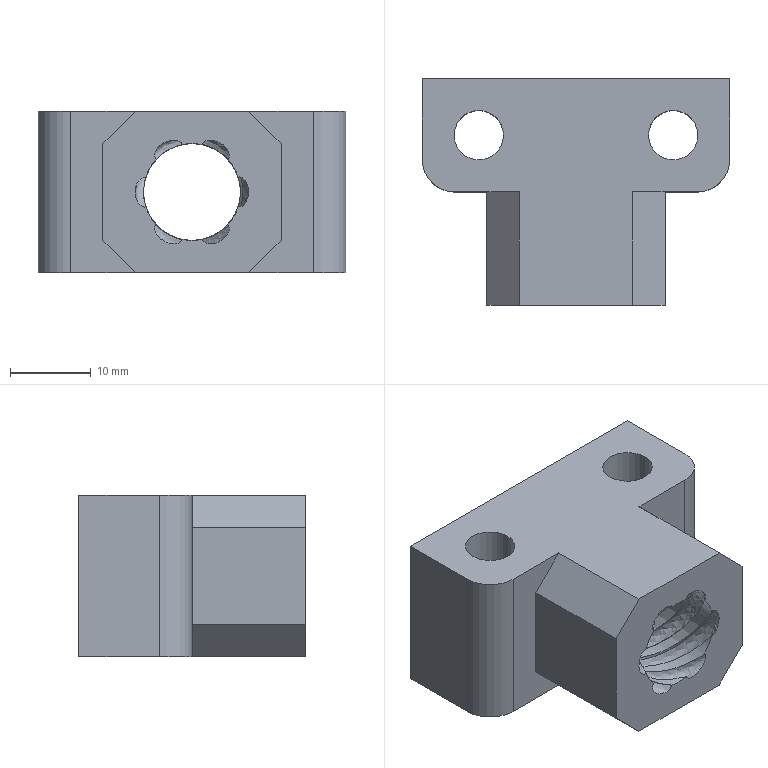Part | NX | features BREP 1 | 1 solid | 52 faces | volume 11357 mm3 | cylinder 26 | plane 14 | spline 12 | commonest cylinder face diameters 12 x20 6.1 x4 8 x2